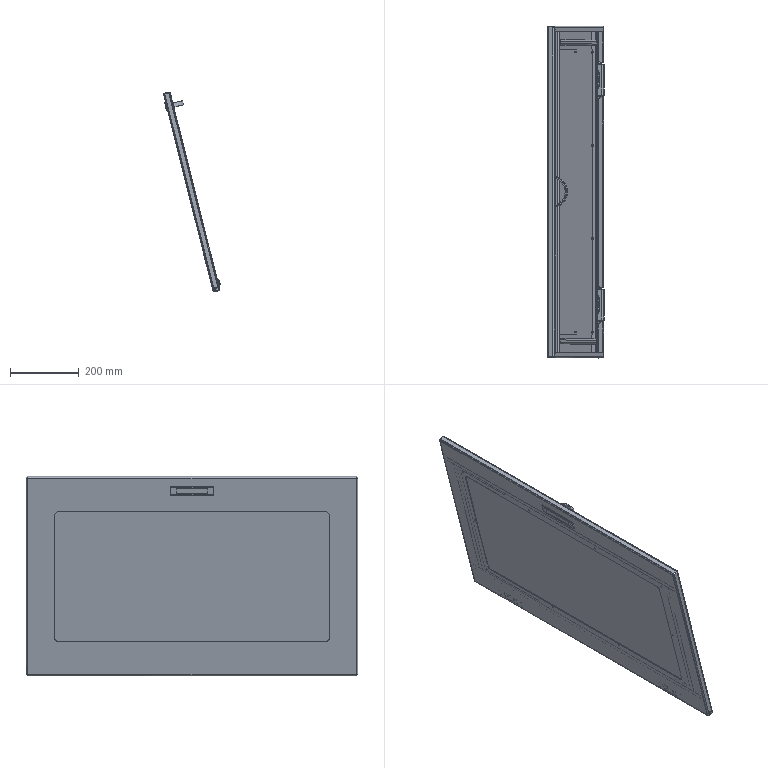Part | NX | features BREP 10 | 12 solids | 594 faces | box 164.614 x 963 x 580.226 mm | volume 2670219 mm3 | plane 296 | cylinder 216 | cone 48 | torus 18 | spline 16 | commonest cylinder face diameters 7 x38 5 x24 4 x20 5.8 x20 12 x18 8 x16